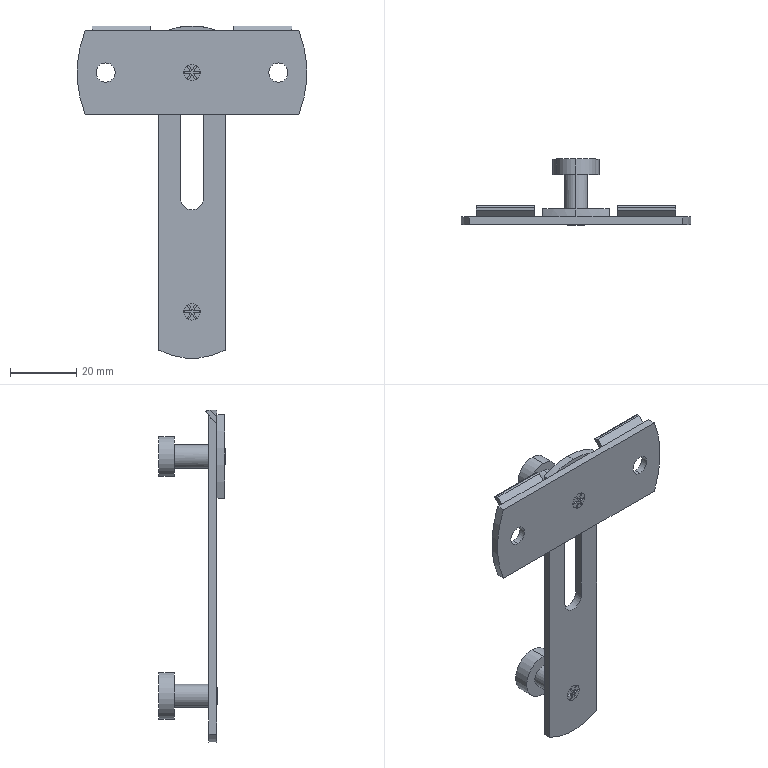Part | SolidWorks | features BaseBody 1 | 1 solid | 95 faces | box 69.2 x 20 x 100 mm | volume 10290 mm3 | plane 55 | cylinder 36 | cone 4 | commonest cylinder face diameters 4.8 x12 7 x5 5 x4 5.8 x4 42.5 x3 1 x2